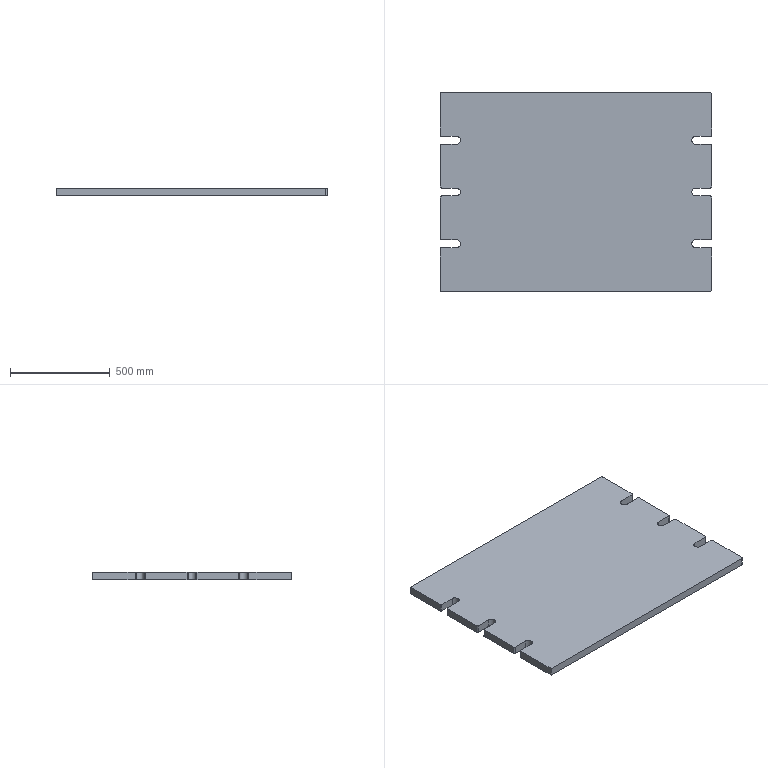Part | SolidWorks | features Fillet 2, Extrusion 1 | 1 solid | 47 faces | box 1360 x 1000 x 40 mm | volume 53476912 mm3 | plane 24 | cylinder 23 | commonest cylinder face diameters 10 x12 40 x9 20 x2
STEP:
#1=CARTESIAN_POINT('',(1260.,760.,40.));
#2=VERTEX_POINT('',#1);
#3=CARTESIAN_POINT('',(1280.,780.,40.));
#4=VERTEX_POINT('',#3);
#5=CARTESIAN_POINT('',(1280.,760.,40.));
#6=DIRECTION('',(0.,0.,-1.));
#7=DIRECTION('',(1.,0.,0.));
#8=AXIS2_PLACEMENT_3D('',#5,#6,#7);
#9=CIRCLE('',#8,20.);
#10=EDGE_CURVE('',#2,#4,#9,.T.);
#11=ORIENTED_EDGE('',*,*,#10,.F.);
#12=CARTESIAN_POINT('',(1260.,760.,0.));
#13=VERTEX_POINT('',#12);
#14=CARTESIAN_POINT('',(1260.,760.,40.));
#15=DIRECTION('',(0.,0.,-1.));
#16=VECTOR('',#15,1000.);
#17=LINE('',#14,#16);
#18=EDGE_CURVE('',#2,#13,#17,.T.);
#19=ORIENTED_EDGE('',*,*,#18,.T.);
#20=CARTESIAN_POINT('',(1280.,780.,0.));
#21=VERTEX_POINT('',#20);
#22=CARTESIAN_POINT('',(1280.,760.,0.));
#23=DIRECTION('',(0.,0.,-1.));
#24=DIRECTION('',(1.,0.,0.));
#25=AXIS2_PLACEMENT_3D('',#22,#23,#24);
#26=CIRCLE('',#25,20.);
#27=EDGE_CURVE('',#13,#21,#26,.T.);
#28=ORIENTED_EDGE('',*,*,#27,.T.);
#29=CARTESIAN_POINT('',(1280.,780.,40.));
#30=DIRECTION('',(0.,0.,-1.));
#31=VECTOR('',#30,1000.);
#32=LINE('',#29,#31);
#33=EDGE_CURVE('',#4,#21,#32,.T.);
#34=ORIENTED_EDGE('',*,*,#33,.F.);
#35=EDGE_LOOP('',(#11,#19,#28,#34));
#36=FACE_OUTER_BOUND('',#35,.T.);
#37=CARTESIAN_POINT('',(1280.,760.,40.));
#38=DIRECTION('',(0.,0.,-1.));
#39=DIRECTION('',(-1.,0.,0.));
#40=AXIS2_PLACEMENT_3D('',#37,#38,#39);
#41=CYLINDRICAL_SURFACE('',#40,20.);
#42=ADVANCED_FACE('',(#36),#41,.F.);
#43=CARTESIAN_POINT('',(1260.,500.,40.));
#44=VERTEX_POINT('',#43);
#45=CARTESIAN_POINT('',(1280.,520.,40.));
#46=VERTEX_POINT('',#45);
#47=CARTESIAN_POINT('',(1280.,500.,40.));
#48=DIRECTION('',(0.,0.,-1.));
#49=DIRECTION('',(1.,0.,0.));
#50=AXIS2_PLACEMENT_3D('',#47,#48,#49);
#51=CIRCLE('',#50,20.);
#52=EDGE_CURVE('',#44,#46,#51,.T.);
#53=ORIENTED_EDGE('',*,*,#52,.F.);
#54=CARTESIAN_POINT('',(1260.,500.,0.));
#55=VERTEX_POINT('',#54);
#56=CARTESIAN_POINT('',(1260.,500.,40.));
#57=DIRECTION('',(0.,0.,-1.));
#58=VECTOR('',#57,1000.);
#59=LINE('',#56,#58);
#60=EDGE_CURVE('',#44,#55,#59,.T.);
#61=ORIENTED_EDGE('',*,*,#60,.T.);
#62=CARTESIAN_POINT('',(1280.,520.,0.));
#63=VERTEX_POINT('',#62);
#64=CARTESIAN_POINT('',(1280.,500.,0.));
#65=DIRECTION('',(0.,0.,-1.));
#66=DIRECTION('',(1.,0.,0.));
#67=AXIS2_PLACEMENT_3D('',#64,#65,#66);
#68=CIRCLE('',#67,20.);
#69=EDGE_CURVE('',#55,#63,#68,.T.);
#70=ORIENTED_EDGE('',*,*,#69,.T.);
#71=CARTESIAN_POINT('',(1280.,520.,40.));
#72=DIRECTION('',(0.,0.,-1.));
#73=VECTOR('',#72,1000.);
#74=LINE('',#71,#73);
#75=EDGE_CURVE('',#46,#63,#74,.T.);
#76=ORIENTED_EDGE('',*,*,#75,.F.);
#77=EDGE_LOOP('',(#53,#61,#70,#76));
#78=FACE_OUTER_BOUND('',#77,.T.);
#79=CARTESIAN_POINT('',(1280.,500.,40.));
#80=DIRECTION('',(0.,0.,-1.));
#81=DIRECTION('',(-1.,0.,0.));
#82=AXIS2_PLACEMENT_3D('',#79,#80,#81);
#83=CYLINDRICAL_SURFACE('',#82,20.);
#84=ADVANCED_FACE('',(#78),#83,.F.);
#85=CARTESIAN_POINT('',(1260.,240.,40.));
#86=VERTEX_POINT('',#85);
#87=CARTESIAN_POINT('',(1280.,260.,40.));
#88=VERTEX_POINT('',#87);
#89=CARTESIAN_POINT('',(1280.,240.,40.));
#90=DIRECTION('',(0.,0.,-1.));
#91=DIRECTION('',(1.,0.,0.));
#92=AXIS2_PLACEMENT_3D('',#89,#90,#91);
#93=CIRCLE('',#92,20.);
#94=EDGE_CURVE('',#86,#88,#93,.T.);
#95=ORIENTED_EDGE('',*,*,#94,.F.);
#96=CARTESIAN_POINT('',(1260.,240.,0.));
#97=VERTEX_POINT('',#96);
#98=CARTESIAN_POINT('',(1260.,240.,40.));
#99=DIRECTION('',(0.,0.,-1.));
#100=VECTOR('',#99,1000.);
#101=LINE('',#98,#100);
#102=EDGE_CURVE('',#86,#97,#101,.T.);
#103=ORIENTED_EDGE('',*,*,#102,.T.);
#104=CARTESIAN_POINT('',(1280.,260.,0.));
#105=VERTEX_POINT('',#104);
#106=CARTESIAN_POINT('',(1280.,240.,0.));
#107=DIRECTION('',(0.,0.,-1.));
#108=DIRECTION('',(1.,0.,0.));
#109=AXIS2_PLACEMENT_3D('',#106,#107,#108);
#110=CIRCLE('',#109,20.);
#111=EDGE_CURVE('',#97,#105,#110,.T.);
#112=ORIENTED_EDGE('',*,*,#111,.T.);
#113=CARTESIAN_POINT('',(1280.,260.,40.));
#114=DIRECTION('',(0.,0.,-1.));
#115=VECTOR('',#114,1000.);
#116=LINE('',#113,#115);
#117=EDGE_CURVE('',#88,#105,#116,.T.);
#118=ORIENTED_EDGE('',*,*,#117,.F.);
#119=EDGE_LOOP('',(#95,#103,#112,#118));
#120=FACE_OUTER_BOUND('',#119,.T.);
#121=CARTESIAN_POINT('',(1280.,240.,40.));
#122=DIRECTION('',(0.,0.,-1.));
#123=DIRECTION('',(-1.,0.,0.));
#124=AXIS2_PLACEMENT_3D('',#121,#122,#123);
#125=CYLINDRICAL_SURFACE('',#124,20.);
#126=ADVANCED_FACE('',(#120),#125,.F.);
#127=CARTESIAN_POINT('',(0.,215.,40.));
#128=VERTEX_POINT('',#127);
#129=CARTESIAN_POINT('',(0.,0.,40.));
#130=VERTEX_POINT('',#129);
#131=CARTESIAN_POINT('',(0.,0.,40.));
#132=DIRECTION('',(0.,-1.,0.));
#133=VECTOR('',#132,1000.);
#134=LINE('',#131,#133);
#135=EDGE_CURVE('',#128,#130,#134,.T.);
#136=ORIENTED_EDGE('',*,*,#135,.F.);
#137=CARTESIAN_POINT('',(0.,215.,0.));
#138=VERTEX_POINT('',#137);
#139=CARTESIAN_POINT('',(0.,215.,40.));
#140=DIRECTION('',(0.,0.,-1.));
#141=VECTOR('',#140,1000.);
#142=LINE('',#139,#141);
#143=EDGE_CURVE('',#128,#138,#142,.T.);
#144=ORIENTED_EDGE('',*,*,#143,.T.);
#145=CARTESIAN_POINT('',(0.,0.,0.));
#146=VERTEX_POINT('',#145);
#147=CARTESIAN_POINT('',(0.,0.,0.));
#148=DIRECTION('',(0.,-1.,0.));
#149=VECTOR('',#148,1000.);
#150=LINE('',#147,#149);
#151=EDGE_CURVE('',#138,#146,#150,.T.);
#152=ORIENTED_EDGE('',*,*,#151,.T.);
#153=CARTESIAN_POINT('',(0.,0.,40.));
#154=DIRECTION('',(0.,0.,-1.));
#155=VECTOR('',#154,1000.);
#156=LINE('',#153,#155);
#157=EDGE_CURVE('',#130,#146,#156,.T.);
#158=ORIENTED_EDGE('',*,*,#157,.F.);
#159=EDGE_LOOP('',(#136,#144,#152,#158));
#160=FACE_OUTER_BOUND('',#159,.T.);
#161=CARTESIAN_POINT('',(0.,0.,40.));
#162=DIRECTION('',(1.,0.,0.));
#163=DIRECTION('',(0.,1.,0.));
#164=AXIS2_PLACEMENT_3D('',#161,#162,#163);
#165=PLANE('',#164);
#166=ADVANCED_FACE('',(#160),#165,.F.);
#167=CARTESIAN_POINT('',(1350.,0.,0.));
#168=VERTEX_POINT('',#167);
#169=CARTESIAN_POINT('',(0.,0.,0.));
#170=DIRECTION('',(1.,0.,0.));
#171=VECTOR('',#170,1000.);
#172=LINE('',#169,#171);
#173=EDGE_CURVE('',#146,#168,#172,.T.);
#174=ORIENTED_EDGE('',*,*,#173,.T.);
#175=CARTESIAN_POINT('',(1350.,0.,40.));
#176=VERTEX_POINT('',#175);
#177=CARTESIAN_POINT('',(1350.,0.,40.));
#178=DIRECTION('',(0.,0.,1.));
#179=VECTOR('',#178,1000.);
#180=LINE('',#177,#179);
#181=EDGE_CURVE('',#168,#176,#180,.T.);
#182=ORIENTED_EDGE('',*,*,#181,.T.);
#183=CARTESIAN_POINT('',(0.,0.,40.));
#184=DIRECTION('',(1.,0.,0.));
#185=VECTOR('',#184,1000.);
#186=LINE('',#183,#185);
#187=EDGE_CURVE('',#130,#176,#186,.T.);
#188=ORIENTED_EDGE('',*,*,#187,.F.);
#189=ORIENTED_EDGE('',*,*,#157,.T.);
#190=EDGE_LOOP('',(#174,#182,#188,#189));
#191=FACE_OUTER_BOUND('',#190,.T.);
#192=CARTESIAN_POINT('',(0.,0.,40.));
#193=DIRECTION('',(0.,1.,0.));
#194=DIRECTION('',(0.,0.,1.));
#195=AXIS2_PLACEMENT_3D('',#192,#193,#194);
#196=PLANE('',#195);
#197=ADVANCED_FACE('',(#191),#196,.F.);
#198=CARTESIAN_POINT('',(1360.,10.,40.));
#199=VERTEX_POINT('',#198);
#200=CARTESIAN_POINT('',(1360.,215.,40.));
#201=VERTEX_POINT('',#200);
#202=CARTESIAN_POINT('',(1360.,0.,40.));
#203=DIRECTION('',(0.,1.,0.));
#204=VECTOR('',#203,1000.);
#205=LINE('',#202,#204);
#206=EDGE_CURVE('',#199,#201,#205,.T.);
#207=ORIENTED_EDGE('',*,*,#206,.F.);
#208=CARTESIAN_POINT('',(1360.,10.,0.));
#209=VERTEX_POINT('',#208);
#210=CARTESIAN_POINT('',(1360.,10.,40.));
#211=DIRECTION('',(0.,0.,-1.));
#212=VECTOR('',#211,1000.);
#213=LINE('',#210,#212);
#214=EDGE_CURVE('',#199,#209,#213,.T.);
#215=ORIENTED_EDGE('',*,*,#214,.T.);
#216=CARTESIAN_POINT('',(1360.,215.,0.));
#217=VERTEX_POINT('',#216);
#218=CARTESIAN_POINT('',(1360.,0.,0.));
#219=DIRECTION('',(0.,1.,0.));
#220=VECTOR('',#219,1000.);
#221=LINE('',#218,#220);
#222=EDGE_CURVE('',#209,#217,#221,.T.);
#223=ORIENTED_EDGE('',*,*,#222,.T.);
#224=CARTESIAN_POINT('',(1360.,215.,40.));
#225=DIRECTION('',(0.,0.,1.));
#226=VECTOR('',#225,1000.);
#227=LINE('',#224,#226);
#228=EDGE_CURVE('',#217,#201,#227,.T.);
#229=ORIENTED_EDGE('',*,*,#228,.T.);
#230=EDGE_LOOP('',(#207,#215,#223,#229));
#231=FACE_OUTER_BOUND('',#230,.T.);
#232=CARTESIAN_POINT('',(1360.,0.,40.));
#233=DIRECTION('',(-1.,0.,0.));
#234=DIRECTION('',(0.,0.,1.));
#235=AXIS2_PLACEMENT_3D('',#232,#233,#234);
#236=PLANE('',#235);
#237=ADVANCED_FACE('',(#231),#236,.F.);
#238=CARTESIAN_POINT('',(1355.,220.,40.));
#239=VERTEX_POINT('',#238);
#240=CARTESIAN_POINT('',(1280.,220.,40.));
#241=VERTEX_POINT('',#240);
#242=CARTESIAN_POINT('',(1280.,220.,40.));
#243=DIRECTION('',(-1.,0.,0.));
#244=VECTOR('',#243,1000.);
#245=LINE('',#242,#244);
#246=EDGE_CURVE('',#239,#241,#245,.T.);
#247=ORIENTED_EDGE('',*,*,#246,.F.);
#248=CARTESIAN_POINT('',(1355.,220.,0.));
#249=VERTEX_POINT('',#248);
#250=CARTESIAN_POINT('',(1355.,220.,40.));
#251=DIRECTION('',(0.,0.,-1.));
#252=VECTOR('',#251,1000.);
#253=LINE('',#250,#252);
#254=EDGE_CURVE('',#239,#249,#253,.T.);
#255=ORIENTED_EDGE('',*,*,#254,.T.);
#256=CARTESIAN_POINT('',(1280.,220.,0.));
#257=VERTEX_POINT('',#256);
#258=CARTESIAN_POINT('',(1280.,220.,0.));
#259=DIRECTION('',(-1.,0.,0.));
#260=VECTOR('',#259,1000.);
#261=LINE('',#258,#260);
#262=EDGE_CURVE('',#249,#257,#261,.T.);
#263=ORIENTED_EDGE('',*,*,#262,.T.);
#264=CARTESIAN_POINT('',(1280.,220.,40.));
#265=DIRECTION('',(0.,0.,-1.));
#266=VECTOR('',#265,1000.);
#267=LINE('',#264,#266);
#268=EDGE_CURVE('',#241,#257,#267,.T.);
#269=ORIENTED_EDGE('',*,*,#268,.F.);
#270=EDGE_LOOP('',(#247,#255,#263,#269));
#271=FACE_OUTER_BOUND('',#270,.T.);
#272=CARTESIAN_POINT('',(1280.,220.,40.));
#273=DIRECTION('',(0.,-1.,0.));
#274=DIRECTION('',(1.,0.,0.));
#275=AXIS2_PLACEMENT_3D('',#272,#273,#274);
#276=PLANE('',#275);
#277=ADVANCED_FACE('',(#271),#276,.F.);
#278=ORIENTED_EDGE('',*,*,#102,.F.);
#279=CARTESIAN_POINT('',(1280.,240.,40.));
#280=DIRECTION('',(0.,0.,-1.));
#281=DIRECTION('',(1.,0.,0.));
#282=AXIS2_PLACEMENT_3D('',#279,#280,#281);
#283=CIRCLE('',#282,20.);
#284=EDGE_CURVE('',#241,#86,#283,.T.);
#285=ORIENTED_EDGE('',*,*,#284,.F.);
#286=ORIENTED_EDGE('',*,*,#268,.T.);
#287=CARTESIAN_POINT('',(1280.,240.,0.));
#288=DIRECTION('',(0.,0.,-1.));
#289=DIRECTION('',(1.,0.,0.));
#290=AXIS2_PLACEMENT_3D('',#287,#288,#289);
#291=CIRCLE('',#290,20.);
#292=EDGE_CURVE('',#257,#97,#291,.T.);
#293=ORIENTED_EDGE('',*,*,#292,.T.);
#294=EDGE_LOOP('',(#278,#285,#286,#293));
#295=FACE_OUTER_BOUND('',#294,.T.);
#296=CARTESIAN_POINT('',(1280.,240.,40.));
#297=DIRECTION('',(0.,0.,-1.));
#298=DIRECTION('',(-1.,0.,0.));
#299=AXIS2_PLACEMENT_3D('',#296,#297,#298);
#300=CYLINDRICAL_SURFACE('',#299,20.);
#301=ADVANCED_FACE('',(#295),#300,.F.);
#302=CARTESIAN_POINT('',(1355.,260.,0.));
#303=VERTEX_POINT('',#302);
#304=CARTESIAN_POINT('',(1360.,260.,0.));
#305=DIRECTION('',(1.,0.,0.));
#306=VECTOR('',#305,1000.);
#307=LINE('',#304,#306);
#308=EDGE_CURVE('',#105,#303,#307,.T.);
#309=ORIENTED_EDGE('',*,*,#308,.T.);
#310=CARTESIAN_POINT('',(1355.,260.,40.));
#311=VERTEX_POINT('',#310);
#312=CARTESIAN_POINT('',(1355.,260.,40.));
#313=DIRECTION('',(0.,0.,1.));
#314=VECTOR('',#313,1000.);
#315=LINE('',#312,#314);
#316=EDGE_CURVE('',#303,#311,#315,.T.);
#317=ORIENTED_EDGE('',*,*,#316,.T.);
#318=CARTESIAN_POINT('',(1360.,260.,40.));
#319=DIRECTION('',(1.,0.,0.));
#320=VECTOR('',#319,1000.);
#321=LINE('',#318,#320);
#322=EDGE_CURVE('',#88,#311,#321,.T.);
#323=ORIENTED_EDGE('',*,*,#322,.F.);
#324=ORIENTED_EDGE('',*,*,#117,.T.);
#325=EDGE_LOOP('',(#309,#317,#323,#324));
#326=FACE_OUTER_BOUND('',#325,.T.);
#327=CARTESIAN_POINT('',(1360.,260.,40.));
#328=DIRECTION('',(0.,1.,0.));
#329=DIRECTION('',(0.,0.,1.));
#330=AXIS2_PLACEMENT_3D('',#327,#328,#329);
#331=PLANE('',#330);
#332=ADVANCED_FACE('',(#326),#331,.F.);
#333=CARTESIAN_POINT('',(1360.,265.,0.));
#334=VERTEX_POINT('',#333);
#335=CARTESIAN_POINT('',(1360.,475.,0.));
#336=VERTEX_POINT('',#335);
#337=CARTESIAN_POINT('',(1360.,260.,0.));
#338=DIRECTION('',(0.,1.,0.));
#339=VECTOR('',#338,1000.);
#340=LINE('',#337,#339);
#341=EDGE_CURVE('',#334,#336,#340,.T.);
#342=ORIENTED_EDGE('',*,*,#341,.T.);
#343=CARTESIAN_POINT('',(1360.,475.,40.));
#344=VERTEX_POINT('',#343);
#345=CARTESIAN_POINT('',(1360.,475.,40.));
#346=DIRECTION('',(0.,0.,1.));
#347=VECTOR('',#346,1000.);
#348=LINE('',#345,#347);
#349=EDGE_CURVE('',#336,#344,#348,.T.);
#350=ORIENTED_EDGE('',*,*,#349,.T.);
#351=CARTESIAN_POINT('',(1360.,265.,40.));
#352=VERTEX_POINT('',#351);
#353=CARTESIAN_POINT('',(1360.,260.,40.));
#354=DIRECTION('',(0.,1.,0.));
#355=VECTOR('',#354,1000.);
#356=LINE('',#353,#355);
#357=EDGE_CURVE('',#352,#344,#356,.T.);
#358=ORIENTED_EDGE('',*,*,#357,.F.);
#359=CARTESIAN_POINT('',(1360.,265.,40.));
#360=DIRECTION('',(0.,0.,-1.));
#361=VECTOR('',#360,1000.);
#362=LINE('',#359,#361);
#363=EDGE_CURVE('',#352,#334,#362,.T.);
#364=ORIENTED_EDGE('',*,*,#363,.T.);
#365=EDGE_LOOP('',(#342,#350,#358,#364));
#366=FACE_OUTER_BOUND('',#365,.T.);
#367=CARTESIAN_POINT('',(1360.,260.,40.));
#368=DIRECTION('',(-1.,0.,0.));
#369=DIRECTION('',(0.,0.,1.));
#370=AXIS2_PLACEMENT_3D('',#367,#368,#369);
#371=PLANE('',#370);
#372=ADVANCED_FACE('',(#366),#371,.F.);
#373=CARTESIAN_POINT('',(1355.,480.,40.));
#374=VERTEX_POINT('',#373);
#375=CARTESIAN_POINT('',(1280.,480.,40.));
#376=VERTEX_POINT('',#375);
#377=CARTESIAN_POINT('',(1280.,480.,40.));
#378=DIRECTION('',(-1.,0.,0.));
#379=VECTOR('',#378,1000.);
#380=LINE('',#377,#379);
#381=EDGE_CURVE('',#374,#376,#380,.T.);
#382=ORIENTED_EDGE('',*,*,#381,.F.);
#383=CARTESIAN_POINT('',(1355.,480.,0.));
#384=VERTEX_POINT('',#383);
#385=CARTESIAN_POINT('',(1355.,480.,40.));
#386=DIRECTION('',(0.,0.,-1.));
#387=VECTOR('',#386,1000.);
#388=LINE('',#385,#387);
#389=EDGE_CURVE('',#374,#384,#388,.T.);
#390=ORIENTED_EDGE('',*,*,#389,.T.);
#391=CARTESIAN_POINT('',(1280.,480.,0.));
#392=VERTEX_POINT('',#391);
#393=CARTESIAN_POINT('',(1280.,480.,0.));
#394=DIRECTION('',(-1.,0.,0.));
#395=VECTOR('',#394,1000.);
#396=LINE('',#393,#395);
#397=EDGE_CURVE('',#384,#392,#396,.T.);
#398=ORIENTED_EDGE('',*,*,#397,.T.);
#399=CARTESIAN_POINT('',(1280.,480.,40.));
#400=DIRECTION('',(0.,0.,-1.));
#401=VECTOR('',#400,1000.);
#402=LINE('',#399,#401);
#403=EDGE_CURVE('',#376,#392,#402,.T.);
#404=ORIENTED_EDGE('',*,*,#403,.F.);
#405=EDGE_LOOP('',(#382,#390,#398,#404));
#406=FACE_OUTER_BOUND('',#405,.T.);
#407=CARTESIAN_POINT('',(1280.,480.,40.));
#408=DIRECTION('',(0.,-1.,0.));
#409=DIRECTION('',(1.,0.,0.));
#410=AXIS2_PLACEMENT_3D('',#407,#408,#409);
#411=PLANE('',#410);
#412=ADVANCED_FACE('',(#406),#411,.F.);
#413=ORIENTED_EDGE('',*,*,#60,.F.);
#414=CARTESIAN_POINT('',(1280.,500.,40.));
#415=DIRECTION('',(0.,0.,-1.));
#416=DIRECTION('',(1.,0.,0.));
#417=AXIS2_PLACEMENT_3D('',#414,#415,#416);
#418=CIRCLE('',#417,20.);
#419=EDGE_CURVE('',#376,#44,#418,.T.);
#420=ORIENTED_EDGE('',*,*,#419,.F.);
#421=ORIENTED_EDGE('',*,*,#403,.T.);
#422=CARTESIAN_POINT('',(1280.,500.,0.));
#423=DIRECTION('',(0.,0.,-1.));
#424=DIRECTION('',(1.,0.,0.));
#425=AXIS2_PLACEMENT_3D('',#422,#423,#424);
#426=CIRCLE('',#425,20.);
#427=EDGE_CURVE('',#392,#55,#426,.T.);
#428=ORIENTED_EDGE('',*,*,#427,.T.);
#429=EDGE_LOOP('',(#413,#420,#421,#428));
#430=FACE_OUTER_BOUND('',#429,.T.);
#431=CARTESIAN_POINT('',(1280.,500.,40.));
#432=DIRECTION('',(0.,0.,-1.));
#433=DIRECTION('',(-1.,0.,0.));
#434=AXIS2_PLACEMENT_3D('',#431,#432,#433);
#435=CYLINDRICAL_SURFACE('',#434,20.);
#436=ADVANCED_FACE('',(#430),#435,.F.);
#437=CARTESIAN_POINT('',(1355.,520.,0.));
#438=VERTEX_POINT('',#437);
#439=CARTESIAN_POINT('',(1360.,520.,0.));
#440=DIRECTION('',(1.,0.,0.));
#441=VECTOR('',#440,1000.);
#442=LINE('',#439,#441);
#443=EDGE_CURVE('',#63,#438,#442,.T.);
#444=ORIENTED_EDGE('',*,*,#443,.T.);
#445=CARTESIAN_POINT('',(1355.,520.,40.));
#446=VERTEX_POINT('',#445);
#447=CARTESIAN_POINT('',(1355.,520.,40.));
#448=DIRECTION('',(0.,0.,1.));
#449=VECTOR('',#448,1000.);
#450=LINE('',#447,#449);
#451=EDGE_CURVE('',#438,#446,#450,.T.);
#452=ORIENTED_EDGE('',*,*,#451,.T.);
#453=CARTESIAN_POINT('',(1360.,520.,40.));
#454=DIRECTION('',(1.,0.,0.));
#455=VECTOR('',#454,1000.);
#456=LINE('',#453,#455);
#457=EDGE_CURVE('',#46,#446,#456,.T.);
#458=ORIENTED_EDGE('',*,*,#457,.F.);
#459=ORIENTED_EDGE('',*,*,#75,.T.);
#460=EDGE_LOOP('',(#444,#452,#458,#459));
#461=FACE_OUTER_BOUND('',#460,.T.);
#462=CARTESIAN_POINT('',(1360.,520.,40.));
#463=DIRECTION('',(0.,1.,0.));
#464=DIRECTION('',(0.,0.,1.));
#465=AXIS2_PLACEMENT_3D('',#462,#463,#464);
#466=PLANE('',#465);
#467=ADVANCED_FACE('',(#461),#466,.F.);
#468=CARTESIAN_POINT('',(1360.,525.,0.));
#469=VERTEX_POINT('',#468);
#470=CARTESIAN_POINT('',(1360.,735.,0.));
#471=VERTEX_POINT('',#470);
#472=CARTESIAN_POINT('',(1360.,520.,0.));
#473=DIRECTION('',(0.,1.,0.));
#474=VECTOR('',#473,1000.);
#475=LINE('',#472,#474);
#476=EDGE_CURVE('',#469,#471,#475,.T.);
#477=ORIENTED_EDGE('',*,*,#476,.T.);
#478=CARTESIAN_POINT('',(1360.,735.,40.));
#479=VERTEX_POINT('',#478);
#480=CARTESIAN_POINT('',(1360.,735.,40.));
#481=DIRECTION('',(0.,0.,1.));
#482=VECTOR('',#481,1000.);
#483=LINE('',#480,#482);
#484=EDGE_CURVE('',#471,#479,#483,.T.);
#485=ORIENTED_EDGE('',*,*,#484,.T.);
#486=CARTESIAN_POINT('',(1360.,525.,40.));
#487=VERTEX_POINT('',#486);
#488=CARTESIAN_POINT('',(1360.,520.,40.));
#489=DIRECTION('',(0.,1.,0.));
#490=VECTOR('',#489,1000.);
#491=LINE('',#488,#490);
#492=EDGE_CURVE('',#487,#479,#491,.T.);
#493=ORIENTED_EDGE('',*,*,#492,.F.);
#494=CARTESIAN_POINT('',(1360.,525.,40.));
#495=DIRECTION('',(0.,0.,-1.));
#496=VECTOR('',#495,1000.);
#497=LINE('',#494,#496);
#498=EDGE_CURVE('',#487,#469,#497,.T.);
#499=ORIENTED_EDGE('',*,*,#498,.T.);
#500=EDGE_LOOP('',(#477,#485,#493,#499));
#501=FACE_OUTER_BOUND('',#500,.T.);
#502=CARTESIAN_POINT('',(1360.,520.,40.));
#503=DIRECTION('',(-1.,0.,0.));
#504=DIRECTION('',(0.,0.,1.));
#505=AXIS2_PLACEMENT_3D('',#502,#503,#504);
#506=PLANE('',#505);
#507=ADVANCED_FACE('',(#501),#506,.F.);
#508=CARTESIAN_POINT('',(1355.,740.,40.));
#509=VERTEX_POINT('',#508);
#510=CARTESIAN_POINT('',(1280.,740.,40.));
#511=VERTEX_POINT('',#510);
#512=CARTESIAN_POINT('',(1280.,740.,40.));
#513=DIRECTION('',(-1.,0.,0.));
#514=VECTOR('',#513,1000.);
#515=LINE('',#512,#514);
#516=EDGE_CURVE('',#509,#511,#515,.T.);
#517=ORIENTED_EDGE('',*,*,#516,.F.);
#518=CARTESIAN_POINT('',(1355.,740.,0.));
#519=VERTEX_POINT('',#518);
#520=CARTESIAN_POINT('',(1355.,740.,40.));
#521=DIRECTION('',(0.,0.,-1.));
#522=VECTOR('',#521,1000.);
#523=LINE('',#520,#522);
#524=EDGE_CURVE('',#509,#519,#523,.T.);
#525=ORIENTED_EDGE('',*,*,#524,.T.);
#526=CARTESIAN_POINT('',(1280.,740.,0.));
#527=VERTEX_POINT('',#526);
#528=CARTESIAN_POINT('',(1280.,740.,0.));
#529=DIRECTION('',(-1.,0.,0.));
#530=VECTOR('',#529,1000.);
#531=LINE('',#528,#530);
#532=EDGE_CURVE('',#519,#527,#531,.T.);
#533=ORIENTED_EDGE('',*,*,#532,.T.);
#534=CARTESIAN_POINT('',(1280.,740.,40.));
#535=DIRECTION('',(0.,0.,-1.));
#536=VECTOR('',#535,1000.);
#537=LINE('',#534,#536);
#538=EDGE_CURVE('',#511,#527,#537,.T.);
#539=ORIENTED_EDGE('',*,*,#538,.F.);
#540=EDGE_LOOP('',(#517,#525,#533,#539));
#541=FACE_OUTER_BOUND('',#540,.T.);
#542=CARTESIAN_POINT('',(1280.,740.,40.));
#543=DIRECTION('',(0.,-1.,0.));
#544=DIRECTION('',(1.,0.,0.));
#545=AXIS2_PLACEMENT_3D('',#542,#543,#544);
#546=PLANE('',#545);
#547=ADVANCED_FACE('',(#541),#546,.F.);
#548=ORIENTED_EDGE('',*,*,#18,.F.);
#549=CARTESIAN_POINT('',(1280.,760.,40.));
#550=DIRECTION('',(0.,0.,-1.));
#551=DIRECTION('',(1.,0.,0.));
#552=AXIS2_PLACEMENT_3D('',#549,#550,#551);
#553=CIRCLE('',#552,20.);
#554=EDGE_CURVE('',#511,#2,#553,.T.);
#555=ORIENTED_EDGE('',*,*,#554,.F.);
#556=ORIENTED_EDGE('',*,*,#538,.T.);
#557=CARTESIAN_POINT('',(1280.,760.,0.));
#558=DIRECTION('',(0.,0.,-1.));
#559=DIRECTION('',(1.,0.,0.));
#560=AXIS2_PLACEMENT_3D('',#557,#558,#559);
#561=CIRCLE('',#560,20.);
#562=EDGE_CURVE('',#527,#13,#561,.T.);
#563=ORIENTED_EDGE('',*,*,#562,.T.);
#564=EDGE_LOOP('',(#548,#555,#556,#563));
#565=FACE_OUTER_BOUND('',#564,.T.);
#566=CARTESIAN_POINT('',(1280.,760.,40.));
#567=DIRECTION('',(0.,0.,-1.));
#568=DIRECTION('',(-1.,0.,0.));
#569=AXIS2_PLACEMENT_3D('',#566,#567,#568);
#570=CYLINDRICAL_SURFACE('',#569,20.);
#571=ADVANCED_FACE('',(#565),#570,.F.);
#572=CARTESIAN_POINT('',(1355.,780.,0.));
#573=VERTEX_POINT('',#572);
#574=CARTESIAN_POINT('',(1360.,780.,0.));
#575=DIRECTION('',(1.,0.,0.));
#576=VECTOR('',#575,1000.);
#577=LINE('',#574,#576);
#578=EDGE_CURVE('',#21,#573,#577,.T.);
#579=ORIENTED_EDGE('',*,*,#578,.T.);
#580=CARTESIAN_POINT('',(1355.,780.,40.));
#581=VERTEX_POINT('',#580);
#582=CARTESIAN_POINT('',(1355.,780.,40.));
#583=DIRECTION('',(0.,0.,1.));
#584=VECTOR('',#583,1000.);
#585=LINE('',#582,#584);
#586=EDGE_CURVE('',#573,#581,#585,.T.);
#587=ORIENTED_EDGE('',*,*,#586,.T.);
#588=CARTESIAN_POINT('',(1360.,780.,40.));
#589=DIRECTION('',(1.,0.,0.));
#590=VECTOR('',#589,1000.);
#591=LINE('',#588,#590);
#592=EDGE_CURVE('',#4,#581,#591,.T.);
#593=ORIENTED_EDGE('',*,*,#592,.F.);
#594=ORIENTED_EDGE('',*,*,#33,.T.);
#595=EDGE_LOOP('',(#579,#587,#593,#594));
#596=FACE_OUTER_BOUND('',#595,.T.);
#597=CARTESIAN_POINT('',(1360.,780.,40.));
#598=DIRECTION('',(0.,1.,0.));
#599=DIRECTION('',(0.,0.,1.));
#600=AXIS2_PLACEMENT_3D('',#597,#598,#599);
#601=PLANE('',#600);
#602=ADVANCED_FACE('',(#596),#601,.F.);
#603=CARTESIAN_POINT('',(1360.,785.,0.));
#604=VERTEX_POINT('',#603);
#605=CARTESIAN_POINT('',(1360.,990.,0.));
#606=VERTEX_POINT('',#605);
#607=CARTESIAN_POINT('',(1360.,780.,0.));
#608=DIRECTION('',(0.,1.,0.));
#609=VECTOR('',#608,1000.);
#610=LINE('',#607,#609);
#611=EDGE_CURVE('',#604,#606,#610,.T.);
#612=ORIENTED_EDGE('',*,*,#611,.T.);
#613=CARTESIAN_POINT('',(1360.,990.,40.));
#614=VERTEX_POINT('',#613);
#615=CARTESIAN_POINT('',(1360.,990.,40.));
#616=DIRECTION('',(0.,0.,1.));
#617=VECTOR('',#616,1000.);
#618=LINE('',#615,#617);
#619=EDGE_CURVE('',#606,#614,#618,.T.);
#620=ORIENTED_EDGE('',*,*,#619,.T.);
#621=CARTESIAN_POINT('',(1360.,785.,40.));
#622=VERTEX_POINT('',#621);
#623=CARTESIAN_POINT('',(1360.,780.,40.));
#624=DIRECTION('',(0.,1.,0.));
#625=VECTOR('',#624,1000.);
#626=LINE('',#623,#625);
#627=EDGE_CURVE('',#622,#614,#626,.T.);
#628=ORIENTED_EDGE('',*,*,#627,.F.);
#629=CARTESIAN_POINT('',(1360.,785.,40.));
#630=DIRECTION('',(0.,0.,-1.));
#631=VECTOR('',#630,1000.);
#632=LINE('',#629,#631);
#633=EDGE_CURVE('',#622,#604,#632,.T.);
#634=ORIENTED_EDGE('',*,*,#633,.T.);
#635=EDGE_LOOP('',(#612,#620,#628,#634));
#636=FACE_OUTER_BOUND('',#635,.T.);
#637=CARTESIAN_POINT('',(1360.,780.,40.));
#638=DIRECTION('',(-1.,0.,0.));
#639=DIRECTION('',(0.,0.,1.));
#640=AXIS2_PLACEMENT_3D('',#637,#638,#639);
#641=PLANE('',#640);
#642=ADVANCED_FACE('',(#636),#641,.F.);
#643=CARTESIAN_POINT('',(1350.,1000.,40.));
#644=VERTEX_POINT('',#643);
#645=CARTESIAN_POINT('',(0.,1000.,40.));
#646=VERTEX_POINT('',#645);
#647=CARTESIAN_POINT('',(0.,1000.,40.));
#648=DIRECTION('',(-1.,0.,0.));
#649=VECTOR('',#648,1000.);
#650=LINE('',#647,#649);
#651=EDGE_CURVE('',#644,#646,#650,.T.);
#652=ORIENTED_EDGE('',*,*,#651,.F.);
#653=CARTESIAN_POINT('',(1350.,1000.,0.));
#654=VERTEX_POINT('',#653);
#655=CARTESIAN_POINT('',(1350.,1000.,40.));
#656=DIRECTION('',(0.,0.,-1.));
#657=VECTOR('',#656,1000.);
#658=LINE('',#655,#657);
#659=EDGE_CURVE('',#644,#654,#658,.T.);
#660=ORIENTED_EDGE('',*,*,#659,.T.);
#661=CARTESIAN_POINT('',(0.,1000.,0.));
#662=VERTEX_POINT('',#661);
#663=CARTESIAN_POINT('',(0.,1000.,0.));
#664=DIRECTION('',(-1.,0.,0.));
#665=VECTOR('',#664,1000.);
#666=LINE('',#663,#665);
#667=EDGE_CURVE('',#654,#662,#666,.T.);
#668=ORIENTED_EDGE('',*,*,#667,.T.);
#669=CARTESIAN_POINT('',(0.,1000.,40.));
#670=DIRECTION('',(0.,0.,-1.));
#671=VECTOR('',#670,1000.);
#672=LINE('',#669,#671);
#673=EDGE_CURVE('',#646,#662,#672,.T.);
#674=ORIENTED_EDGE('',*,*,#673,.F.);
#675=EDGE_LOOP('',(#652,#660,#668,#674));
#676=FACE_OUTER_BOUND('',#675,.T.);
#677=CARTESIAN_POINT('',(0.,1000.,40.));
#678=DIRECTION('',(0.,-1.,0.));
#679=DIRECTION('',(0.,0.,-1.));
#680=AXIS2_PLACEMENT_3D('',#677,#678,#679);
#681=PLANE('',#680);
#682=ADVANCED_FACE('',(#676),#681,.F.);
#683=CARTESIAN_POINT('',(0.,785.,0.));
#684=VERTEX_POINT('',#683);
#685=CARTESIAN_POINT('',(0.,780.,0.));
#686=DIRECTION('',(0.,-1.,0.));
#687=VECTOR('',#686,1000.);
#688=LINE('',#685,#687);
#689=EDGE_CURVE('',#662,#684,#688,.T.);
#690=ORIENTED_EDGE('',*,*,#689,.T.);
#691=CARTESIAN_POINT('',(0.,785.,40.));
#692=VERTEX_POINT('',#691);
#693=CARTESIAN_POINT('',(0.,785.,40.));
#694=DIRECTION('',(0.,0.,1.));
#695=VECTOR('',#694,1000.);
#696=LINE('',#693,#695);
#697=EDGE_CURVE('',#684,#692,#696,.T.);
#698=ORIENTED_EDGE('',*,*,#697,.T.);
#699=CARTESIAN_POINT('',(0.,780.,40.));
#700=DIRECTION('',(0.,-1.,0.));
#701=VECTOR('',#700,1000.);
#702=LINE('',#699,#701);
#703=EDGE_CURVE('',#646,#692,#702,.T.);
#704=ORIENTED_EDGE('',*,*,#703,.F.);
#705=ORIENTED_EDGE('',*,*,#673,.T.);
#706=EDGE_LOOP('',(#690,#698,#704,#705));
#707=FACE_OUTER_BOUND('',#706,.T.);
#708=CARTESIAN_POINT('',(0.,780.,40.));
#709=DIRECTION('',(1.,0.,0.));
#710=DIRECTION('',(0.,0.,-1.));
#711=AXIS2_PLACEMENT_3D('',#708,#709,#710);
#712=PLANE('',#711);
#713=ADVANCED_FACE('',(#707),#712,.F.);
#714=CARTESIAN_POINT('',(5.,780.,40.));
#715=VERTEX_POINT('',#714);
#716=CARTESIAN_POINT('',(80.,780.,40.));
#717=VERTEX_POINT('',#716);
#718=CARTESIAN_POINT('',(0.,780.,40.));
#719=DIRECTION('',(1.,0.,0.));
#720=VECTOR('',#719,1000.);
#721=LINE('',#718,#720);
#722=EDGE_CURVE('',#715,#717,#721,.T.);
#723=ORIENTED_EDGE('',*,*,#722,.F.);
#724=CARTESIAN_POINT('',(5.,780.,0.));
#725=VERTEX_POINT('',#724);
#726=CARTESIAN_POINT('',(5.,780.,40.));
#727=DIRECTION('',(0.,0.,-1.));
#728=VECTOR('',#727,1000.);
#729=LINE('',#726,#728);
#730=EDGE_CURVE('',#715,#725,#729,.T.);
#731=ORIENTED_EDGE('',*,*,#730,.T.);
#732=CARTESIAN_POINT('',(80.,780.,0.));
#733=VERTEX_POINT('',#732);
#734=CARTESIAN_POINT('',(0.,780.,0.));
#735=DIRECTION('',(1.,0.,0.));
#736=VECTOR('',#735,1000.);
#737=LINE('',#734,#736);
#738=EDGE_CURVE('',#725,#733,#737,.T.);
#739=ORIENTED_EDGE('',*,*,#738,.T.);
#740=CARTESIAN_POINT('',(80.,780.,40.));
#741=DIRECTION('',(0.,0.,-1.));
#742=VECTOR('',#741,1000.);
#743=LINE('',#740,#742);
#744=EDGE_CURVE('',#717,#733,#743,.T.);
#745=ORIENTED_EDGE('',*,*,#744,.F.);
#746=EDGE_LOOP('',(#723,#731,#739,#745));
#747=FACE_OUTER_BOUND('',#746,.T.);
#748=CARTESIAN_POINT('',(0.,780.,40.));
#749=DIRECTION('',(0.,1.,0.));
#750=DIRECTION('',(0.,0.,1.));
#751=AXIS2_PLACEMENT_3D('',#748,#749,#750);
#752=PLANE('',#751);
#753=ADVANCED_FACE('',(#747),#752,.F.);
#754=CARTESIAN_POINT('',(80.,740.,0.));
#755=VERTEX_POINT('',#754);
#756=CARTESIAN_POINT('',(80.,760.,0.));
#757=DIRECTION('',(0.,0.,-1.));
#758=DIRECTION('',(-1.,0.,0.));
#759=AXIS2_PLACEMENT_3D('',#756,#757,#758);
#760=CIRCLE('',#759,20.);
#761=EDGE_CURVE('',#733,#755,#760,.T.);
#762=ORIENTED_EDGE('',*,*,#761,.T.);
#763=CARTESIAN_POINT('',(80.,740.,40.));
#764=VERTEX_POINT('',#763);
#765=CARTESIAN_POINT('',(80.,740.,40.));
#766=DIRECTION('',(0.,0.,-1.));
#767=VECTOR('',#766,1000.);
#768=LINE('',#765,#767);
#769=EDGE_CURVE('',#764,#755,#768,.T.);
#770=ORIENTED_EDGE('',*,*,#769,.F.);
#771=CARTESIAN_POINT('',(80.,760.,40.));
#772=DIRECTION('',(0.,0.,-1.));
#773=DIRECTION('',(-1.,0.,0.));
#774=AXIS2_PLACEMENT_3D('',#771,#772,#773);
#775=CIRCLE('',#774,20.);
#776=EDGE_CURVE('',#717,#764,#775,.T.);
#777=ORIENTED_EDGE('',*,*,#776,.F.);
#778=ORIENTED_EDGE('',*,*,#744,.T.);
#779=EDGE_LOOP('',(#762,#770,#777,#778));
#780=FACE_OUTER_BOUND('',#779,.T.);
#781=CARTESIAN_POINT('',(80.,760.,40.));
#782=DIRECTION('',(0.,0.,-1.));
#783=DIRECTION('',(-1.,0.,0.));
#784=AXIS2_PLACEMENT_3D('',#781,#782,#783);
#785=CYLINDRICAL_SURFACE('',#784,20.);
#786=ADVANCED_FACE('',(#780),#785,.F.);
#787=CARTESIAN_POINT('',(5.,740.,0.));
#788=VERTEX_POINT('',#787);
#789=CARTESIAN_POINT('',(80.,740.,0.));
#790=DIRECTION('',(-1.,0.,0.));
#791=VECTOR('',#790,1000.);
#792=LINE('',#789,#791);
#793=EDGE_CURVE('',#755,#788,#792,.T.);
#794=ORIENTED_EDGE('',*,*,#793,.T.);
#795=CARTESIAN_POINT('',(5.,740.,40.));
#796=VERTEX_POINT('',#795);
#797=CARTESIAN_POINT('',(5.,740.,40.));
#798=DIRECTION('',(0.,0.,1.));
#799=VECTOR('',#798,1000.);
#800=LINE('',#797,#799);
#801=EDGE_CURVE('',#788,#796,#800,.T.);
#802=ORIENTED_EDGE('',*,*,#801,.T.);
#803=CARTESIAN_POINT('',(80.,740.,40.));
#804=DIRECTION('',(-1.,0.,0.));
#805=VECTOR('',#804,1000.);
#806=LINE('',#803,#805);
#807=EDGE_CURVE('',#764,#796,#806,.T.);
#808=ORIENTED_EDGE('',*,*,#807,.F.);
#809=ORIENTED_EDGE('',*,*,#769,.T.);
#810=EDGE_LOOP('',(#794,#802,#808,#809));
#811=FACE_OUTER_BOUND('',#810,.T.);
#812=CARTESIAN_POINT('',(80.,740.,40.));
#813=DIRECTION('',(0.,-1.,0.));
#814=DIRECTION('',(0.,0.,-1.));
#815=AXIS2_PLACEMENT_3D('',#812,#813,#814);
#816=PLANE('',#815);
#817=ADVANCED_FACE('',(#811),#816,.F.);
#818=CARTESIAN_POINT('',(0.,735.,0.));
#819=VERTEX_POINT('',#818);
#820=CARTESIAN_POINT('',(0.,525.,0.));
#821=VERTEX_POINT('',#820);
#822=CARTESIAN_POINT('',(0.,520.,0.));
#823=DIRECTION('',(0.,-1.,0.));
#824=VECTOR('',#823,1000.);
#825=LINE('',#822,#824);
#826=EDGE_CURVE('',#819,#821,#825,.T.);
#827=ORIENTED_EDGE('',*,*,#826,.T.);
#828=CARTESIAN_POINT('',(0.,525.,40.));
#829=VERTEX_POINT('',#828);
#830=CARTESIAN_POINT('',(0.,525.,40.));
#831=DIRECTION('',(0.,0.,1.));
#832=VECTOR('',#831,1000.);
#833=LINE('',#830,#832);
#834=EDGE_CURVE('',#821,#829,#833,.T.);
#835=ORIENTED_EDGE('',*,*,#834,.T.);
#836=CARTESIAN_POINT('',(0.,735.,40.));
#837=VERTEX_POINT('',#836);
#838=CARTESIAN_POINT('',(0.,520.,40.));
#839=DIRECTION('',(0.,-1.,0.));
#840=VECTOR('',#839,1000.);
#841=LINE('',#838,#840);
#842=EDGE_CURVE('',#837,#829,#841,.T.);
#843=ORIENTED_EDGE('',*,*,#842,.F.);
#844=CARTESIAN_POINT('',(0.,735.,40.));
#845=DIRECTION('',(0.,0.,-1.));
#846=VECTOR('',#845,1000.);
#847=LINE('',#844,#846);
#848=EDGE_CURVE('',#837,#819,#847,.T.);
#849=ORIENTED_EDGE('',*,*,#848,.T.);
#850=EDGE_LOOP('',(#827,#835,#843,#849));
#851=FACE_OUTER_BOUND('',#850,.T.);
#852=CARTESIAN_POINT('',(0.,520.,40.));
#853=DIRECTION('',(1.,0.,0.));
#854=DIRECTION('',(0.,1.,0.));
#855=AXIS2_PLACEMENT_3D('',#852,#853,#854);
#856=PLANE('',#855);
#857=ADVANCED_FACE('',(#851),#856,.F.);
#858=CARTESIAN_POINT('',(5.,520.,40.));
#859=VERTEX_POINT('',#858);
#860=CARTESIAN_POINT('',(80.,520.,40.));
#861=VERTEX_POINT('',#860);
#862=CARTESIAN_POINT('',(0.,520.,40.));
#863=DIRECTION('',(1.,0.,0.));
#864=VECTOR('',#863,1000.);
#865=LINE('',#862,#864);
#866=EDGE_CURVE('',#859,#861,#865,.T.);
#867=ORIENTED_EDGE('',*,*,#866,.F.);
#868=CARTESIAN_POINT('',(5.,520.,0.));
#869=VERTEX_POINT('',#868);
#870=CARTESIAN_POINT('',(5.,520.,40.));
#871=DIRECTION('',(0.,0.,-1.));
#872=VECTOR('',#871,1000.);
#873=LINE('',#870,#872);
#874=EDGE_CURVE('',#859,#869,#873,.T.);
#875=ORIENTED_EDGE('',*,*,#874,.T.);
#876=CARTESIAN_POINT('',(80.,520.,0.));
#877=VERTEX_POINT('',#876);
#878=CARTESIAN_POINT('',(0.,520.,0.));
#879=DIRECTION('',(1.,0.,0.));
#880=VECTOR('',#879,1000.);
#881=LINE('',#878,#880);
#882=EDGE_CURVE('',#869,#877,#881,.T.);
#883=ORIENTED_EDGE('',*,*,#882,.T.);
#884=CARTESIAN_POINT('',(80.,520.,40.));
#885=DIRECTION('',(0.,0.,-1.));
#886=VECTOR('',#885,1000.);
#887=LINE('',#884,#886);
#888=EDGE_CURVE('',#861,#877,#887,.T.);
#889=ORIENTED_EDGE('',*,*,#888,.F.);
#890=EDGE_LOOP('',(#867,#875,#883,#889));
#891=FACE_OUTER_BOUND('',#890,.T.);
#892=CARTESIAN_POINT('',(0.,520.,40.));
#893=DIRECTION('',(0.,1.,0.));
#894=DIRECTION('',(0.,0.,1.));
#895=AXIS2_PLACEMENT_3D('',#892,#893,#894);
#896=PLANE('',#895);
#897=ADVANCED_FACE('',(#891),#896,.F.);
#898=CARTESIAN_POINT('',(80.,480.,0.));
#899=VERTEX_POINT('',#898);
#900=CARTESIAN_POINT('',(80.,500.,0.));
#901=DIRECTION('',(0.,0.,-1.));
#902=DIRECTION('',(-1.,0.,0.));
#903=AXIS2_PLACEMENT_3D('',#900,#901,#902);
#904=CIRCLE('',#903,20.);
#905=EDGE_CURVE('',#877,#899,#904,.T.);
#906=ORIENTED_EDGE('',*,*,#905,.T.);
#907=CARTESIAN_POINT('',(80.,480.,40.));
#908=VERTEX_POINT('',#907);
#909=CARTESIAN_POINT('',(80.,480.,40.));
#910=DIRECTION('',(0.,0.,-1.));
#911=VECTOR('',#910,1000.);
#912=LINE('',#909,#911);
#913=EDGE_CURVE('',#908,#899,#912,.T.);
#914=ORIENTED_EDGE('',*,*,#913,.F.);
#915=CARTESIAN_POINT('',(80.,500.,40.));
#916=DIRECTION('',(0.,0.,-1.));
#917=DIRECTION('',(-1.,0.,0.));
#918=AXIS2_PLACEMENT_3D('',#915,#916,#917);
#919=CIRCLE('',#918,20.);
#920=EDGE_CURVE('',#861,#908,#919,.T.);
#921=ORIENTED_EDGE('',*,*,#920,.F.);
#922=ORIENTED_EDGE('',*,*,#888,.T.);
#923=EDGE_LOOP('',(#906,#914,#921,#922));
#924=FACE_OUTER_BOUND('',#923,.T.);
#925=CARTESIAN_POINT('',(80.,500.,40.));
#926=DIRECTION('',(0.,0.,-1.));
#927=DIRECTION('',(-1.,0.,0.));
#928=AXIS2_PLACEMENT_3D('',#925,#926,#927);
#929=CYLINDRICAL_SURFACE('',#928,20.);
#930=ADVANCED_FACE('',(#924),#929,.F.);
#931=CARTESIAN_POINT('',(5.,480.,0.));
#932=VERTEX_POINT('',#931);
#933=CARTESIAN_POINT('',(80.,480.,0.));
#934=DIRECTION('',(-1.,0.,0.));
#935=VECTOR('',#934,1000.);
#936=LINE('',#933,#935);
#937=EDGE_CURVE('',#899,#932,#936,.T.);
#938=ORIENTED_EDGE('',*,*,#937,.T.);
#939=CARTESIAN_POINT('',(5.,480.,40.));
#940=VERTEX_POINT('',#939);
#941=CARTESIAN_POINT('',(5.,480.,40.));
#942=DIRECTION('',(0.,0.,1.));
#943=VECTOR('',#942,1000.);
#944=LINE('',#941,#943);
#945=EDGE_CURVE('',#932,#940,#944,.T.);
#946=ORIENTED_EDGE('',*,*,#945,.T.);
#947=CARTESIAN_POINT('',(80.,480.,40.));
#948=DIRECTION('',(-1.,0.,0.));
#949=VECTOR('',#948,1000.);
#950=LINE('',#947,#949);
#951=EDGE_CURVE('',#908,#940,#950,.T.);
#952=ORIENTED_EDGE('',*,*,#951,.F.);
#953=ORIENTED_EDGE('',*,*,#913,.T.);
#954=EDGE_LOOP('',(#938,#946,#952,#953));
#955=FACE_OUTER_BOUND('',#954,.T.);
#956=CARTESIAN_POINT('',(80.,480.,40.));
#957=DIRECTION('',(0.,-1.,0.));
#958=DIRECTION('',(0.,0.,-1.));
#959=AXIS2_PLACEMENT_3D('',#956,#957,#958);
#960=PLANE('',#959);
#961=ADVANCED_FACE('',(#955),#960,.F.);
#962=CARTESIAN_POINT('',(0.,475.,0.));
#963=VERTEX_POINT('',#962);
#964=CARTESIAN_POINT('',(0.,265.,0.));
#965=VERTEX_POINT('',#964);
#966=CARTESIAN_POINT('',(0.,260.,0.));
#967=DIRECTION('',(0.,-1.,0.));
#968=VECTOR('',#967,1000.);
#969=LINE('',#966,#968);
#970=EDGE_CURVE('',#963,#965,#969,.T.);
#971=ORIENTED_EDGE('',*,*,#970,.T.);
#972=CARTESIAN_POINT('',(0.,265.,40.));
#973=VERTEX_POINT('',#972);
#974=CARTESIAN_POINT('',(0.,265.,40.));
#975=DIRECTION('',(0.,0.,1.));
#976=VECTOR('',#975,1000.);
#977=LINE('',#974,#976);
#978=EDGE_CURVE('',#965,#973,#977,.T.);
#979=ORIENTED_EDGE('',*,*,#978,.T.);
#980=CARTESIAN_POINT('',(0.,475.,40.));
#981=VERTEX_POINT('',#980);
#982=CARTESIAN_POINT('',(0.,260.,40.));
#983=DIRECTION('',(0.,-1.,0.));
#984=VECTOR('',#983,1000.);
#985=LINE('',#982,#984);
#986=EDGE_CURVE('',#981,#973,#985,.T.);
#987=ORIENTED_EDGE('',*,*,#986,.F.);
#988=CARTESIAN_POINT('',(0.,475.,40.));
#989=DIRECTION('',(0.,0.,-1.));
#990=VECTOR('',#989,1000.);
#991=LINE('',#988,#990);
#992=EDGE_CURVE('',#981,#963,#991,.T.);
#993=ORIENTED_EDGE('',*,*,#992,.T.);
#994=EDGE_LOOP('',(#971,#979,#987,#993));
#995=FACE_OUTER_BOUND('',#994,.T.);
#996=CARTESIAN_POINT('',(0.,260.,40.));
#997=DIRECTION('',(1.,0.,0.));
#998=DIRECTION('',(0.,1.,0.));
#999=AXIS2_PLACEMENT_3D('',#996,#997,#998);
#1000=PLANE('',#999);
#1001=ADVANCED_FACE('',(#995),#1000,.F.);
#1002=CARTESIAN_POINT('',(5.,260.,40.));
#1003=VERTEX_POINT('',#1002);
#1004=CARTESIAN_POINT('',(80.,260.,40.));
#1005=VERTEX_POINT('',#1004);
#1006=CARTESIAN_POINT('',(0.,260.,40.));
#1007=DIRECTION('',(1.,0.,0.));
#1008=VECTOR('',#1007,1000.);
#1009=LINE('',#1006,#1008);
#1010=EDGE_CURVE('',#1003,#1005,#1009,.T.);
#1011=ORIENTED_EDGE('',*,*,#1010,.F.);
#1012=CARTESIAN_POINT('',(5.,260.,0.));
#1013=VERTEX_POINT('',#1012);
#1014=CARTESIAN_POINT('',(5.,260.,40.));
#1015=DIRECTION('',(0.,0.,-1.));
#1016=VECTOR('',#1015,1000.);
#1017=LINE('',#1014,#1016);
#1018=EDGE_CURVE('',#1003,#1013,#1017,.T.);
#1019=ORIENTED_EDGE('',*,*,#1018,.T.);
#1020=CARTESIAN_POINT('',(80.,260.,0.));
#1021=VERTEX_POINT('',#1020);
#1022=CARTESIAN_POINT('',(0.,260.,0.));
#1023=DIRECTION('',(1.,0.,0.));
#1024=VECTOR('',#1023,1000.);
#1025=LINE('',#1022,#1024);
#1026=EDGE_CURVE('',#1013,#1021,#1025,.T.);
#1027=ORIENTED_EDGE('',*,*,#1026,.T.);
#1028=CARTESIAN_POINT('',(80.,260.,40.));
#1029=DIRECTION('',(0.,0.,-1.));
#1030=VECTOR('',#1029,1000.);
#1031=LINE('',#1028,#1030);
#1032=EDGE_CURVE('',#1005,#1021,#1031,.T.);
#1033=ORIENTED_EDGE('',*,*,#1032,.F.);
#1034=EDGE_LOOP('',(#1011,#1019,#1027,#1033));
#1035=FACE_OUTER_BOUND('',#1034,.T.);
#1036=CARTESIAN_POINT('',(0.,260.,40.));
#1037=DIRECTION('',(0.,1.,0.));
#1038=DIRECTION('',(0.,0.,1.));
#1039=AXIS2_PLACEMENT_3D('',#1036,#1037,#1038);
#1040=PLANE('',#1039);
#1041=ADVANCED_FACE('',(#1035),#1040,.F.);
#1042=CARTESIAN_POINT('',(80.,220.,0.));
#1043=VERTEX_POINT('',#1042);
#1044=CARTESIAN_POINT('',(80.,240.,0.));
#1045=DIRECTION('',(0.,0.,-1.));
#1046=DIRECTION('',(-1.,0.,0.));
#1047=AXIS2_PLACEMENT_3D('',#1044,#1045,#1046);
#1048=CIRCLE('',#1047,20.);
#1049=EDGE_CURVE('',#1021,#1043,#1048,.T.);
#1050=ORIENTED_EDGE('',*,*,#1049,.T.);
#1051=CARTESIAN_POINT('',(80.,220.,40.));
#1052=VERTEX_POINT('',#1051);
#1053=CARTESIAN_POINT('',(80.,220.,40.));
#1054=DIRECTION('',(0.,0.,-1.));
#1055=VECTOR('',#1054,1000.);
#1056=LINE('',#1053,#1055);
#1057=EDGE_CURVE('',#1052,#1043,#1056,.T.);
#1058=ORIENTED_EDGE('',*,*,#1057,.F.);
#1059=CARTESIAN_POINT('',(80.,240.,40.));
#1060=DIRECTION('',(0.,0.,-1.));
#1061=DIRECTION('',(-1.,0.,0.));
#1062=AXIS2_PLACEMENT_3D('',#1059,#1060,#1061);
#1063=CIRCLE('',#1062,20.);
#1064=EDGE_CURVE('',#1005,#1052,#1063,.T.);
#1065=ORIENTED_EDGE('',*,*,#1064,.F.);
#1066=ORIENTED_EDGE('',*,*,#1032,.T.);
#1067=EDGE_LOOP('',(#1050,#1058,#1065,#1066));
#1068=FACE_OUTER_BOUND('',#1067,.T.);
#1069=CARTESIAN_POINT('',(80.,240.,40.));
#1070=DIRECTION('',(0.,0.,-1.));
#1071=DIRECTION('',(-1.,0.,0.));
#1072=AXIS2_PLACEMENT_3D('',#1069,#1070,#1071);
#1073=CYLINDRICAL_SURFACE('',#1072,20.);
#1074=ADVANCED_FACE('',(#1068),#1073,.F.);
#1075=CARTESIAN_POINT('',(5.,220.,0.));
#1076=VERTEX_POINT('',#1075);
#1077=CARTESIAN_POINT('',(80.,220.,0.));
#1078=DIRECTION('',(-1.,0.,0.));
#1079=VECTOR('',#1078,1000.);
#1080=LINE('',#1077,#1079);
#1081=EDGE_CURVE('',#1043,#1076,#1080,.T.);
#1082=ORIENTED_EDGE('',*,*,#1081,.T.);
#1083=CARTESIAN_POINT('',(5.,220.,40.));
#1084=VERTEX_POINT('',#1083);
#1085=CARTESIAN_POINT('',(5.,220.,40.));
#1086=DIRECTION('',(0.,0.,1.));
#1087=VECTOR('',#1086,1000.);
#1088=LINE('',#1085,#1087);
#1089=EDGE_CURVE('',#1076,#1084,#1088,.T.);
#1090=ORIENTED_EDGE('',*,*,#1089,.T.);
#1091=CARTESIAN_POINT('',(80.,220.,40.));
#1092=DIRECTION('',(-1.,0.,0.));
#1093=VECTOR('',#1092,1000.);
#1094=LINE('',#1091,#1093);
#1095=EDGE_CURVE('',#1052,#1084,#1094,.T.);
#1096=ORIENTED_EDGE('',*,*,#1095,.F.);
#1097=ORIENTED_EDGE('',*,*,#1057,.T.);
#1098=EDGE_LOOP('',(#1082,#1090,#1096,#1097));
#1099=FACE_OUTER_BOUND('',#1098,.T.);
#1100=CARTESIAN_POINT('',(80.,220.,40.));
#1101=DIRECTION('',(0.,-1.,0.));
#1102=DIRECTION('',(0.,0.,-1.));
#1103=AXIS2_PLACEMENT_3D('',#1100,#1101,#1102);
#1104=PLANE('',#1103);
#1105=ADVANCED_FACE('',(#1099),#1104,.F.);
#1106=ORIENTED_EDGE('',*,*,#627,.T.);
#1107=CARTESIAN_POINT('',(1350.,990.,40.));
#1108=DIRECTION('',(0.,0.,1.));
#1109=DIRECTION('',(-1.,0.,0.));
#1110=AXIS2_PLACEMENT_3D('',#1107,#1108,#1109);
#1111=CIRCLE('',#1110,10.);
#1112=EDGE_CURVE('',#614,#644,#1111,.T.);
#1113=ORIENTED_EDGE('',*,*,#1112,.T.);
#1114=ORIENTED_EDGE('',*,*,#651,.T.);
#1115=ORIENTED_EDGE('',*,*,#703,.T.);
#1116=CARTESIAN_POINT('',(5.,785.,40.));
#1117=DIRECTION('',(0.,0.,1.));
#1118=DIRECTION('',(-1.,0.,0.));
#1119=AXIS2_PLACEMENT_3D('',#1116,#1117,#1118);
#1120=CIRCLE('',#1119,5.);
#1121=EDGE_CURVE('',#692,#715,#1120,.T.);
#1122=ORIENTED_EDGE('',*,*,#1121,.T.);
#1123=ORIENTED_EDGE('',*,*,#722,.T.);
#1124=ORIENTED_EDGE('',*,*,#776,.T.);
#1125=ORIENTED_EDGE('',*,*,#807,.T.);
#1126=CARTESIAN_POINT('',(5.,735.,40.));
#1127=DIRECTION('',(0.,0.,1.));
#1128=DIRECTION('',(-1.,0.,0.));
#1129=AXIS2_PLACEMENT_3D('',#1126,#1127,#1128);
#1130=CIRCLE('',#1129,5.);
#1131=EDGE_CURVE('',#796,#837,#1130,.T.);
#1132=ORIENTED_EDGE('',*,*,#1131,.T.);
#1133=ORIENTED_EDGE('',*,*,#842,.T.);
#1134=CARTESIAN_POINT('',(5.,525.,40.));
#1135=DIRECTION('',(0.,0.,1.));
#1136=DIRECTION('',(-1.,0.,0.));
#1137=AXIS2_PLACEMENT_3D('',#1134,#1135,#1136);
#1138=CIRCLE('',#1137,5.);
#1139=EDGE_CURVE('',#829,#859,#1138,.T.);
#1140=ORIENTED_EDGE('',*,*,#1139,.T.);
#1141=ORIENTED_EDGE('',*,*,#866,.T.);
#1142=ORIENTED_EDGE('',*,*,#920,.T.);
#1143=ORIENTED_EDGE('',*,*,#951,.T.);
#1144=CARTESIAN_POINT('',(5.,475.,40.));
#1145=DIRECTION('',(0.,0.,1.));
#1146=DIRECTION('',(-1.,0.,0.));
#1147=AXIS2_PLACEMENT_3D('',#1144,#1145,#1146);
#1148=CIRCLE('',#1147,5.);
#1149=EDGE_CURVE('',#940,#981,#1148,.T.);
#1150=ORIENTED_EDGE('',*,*,#1149,.T.);
#1151=ORIENTED_EDGE('',*,*,#986,.T.);
#1152=CARTESIAN_POINT('',(5.,265.,40.));
#1153=DIRECTION('',(0.,0.,1.));
#1154=DIRECTION('',(-1.,0.,0.));
#1155=AXIS2_PLACEMENT_3D('',#1152,#1153,#1154);
#1156=CIRCLE('',#1155,5.);
#1157=EDGE_CURVE('',#973,#1003,#1156,.T.);
#1158=ORIENTED_EDGE('',*,*,#1157,.T.);
#1159=ORIENTED_EDGE('',*,*,#1010,.T.);
#1160=ORIENTED_EDGE('',*,*,#1064,.T.);
#1161=ORIENTED_EDGE('',*,*,#1095,.T.);
#1162=CARTESIAN_POINT('',(5.,215.,40.));
#1163=DIRECTION('',(0.,0.,1.));
#1164=DIRECTION('',(-1.,0.,0.));
#1165=AXIS2_PLACEMENT_3D('',#1162,#1163,#1164);
#1166=CIRCLE('',#1165,5.);
#1167=EDGE_CURVE('',#1084,#128,#1166,.T.);
#1168=ORIENTED_EDGE('',*,*,#1167,.T.);
#1169=ORIENTED_EDGE('',*,*,#135,.T.);
#1170=ORIENTED_EDGE('',*,*,#187,.T.);
#1171=CARTESIAN_POINT('',(1350.,10.,40.));
#1172=DIRECTION('',(0.,0.,1.));
#1173=DIRECTION('',(-1.,0.,0.));
#1174=AXIS2_PLACEMENT_3D('',#1171,#1172,#1173);
#1175=CIRCLE('',#1174,10.);
#1176=EDGE_CURVE('',#176,#199,#1175,.T.);
#1177=ORIENTED_EDGE('',*,*,#1176,.T.);
#1178=ORIENTED_EDGE('',*,*,#206,.T.);
#1179=CARTESIAN_POINT('',(1355.,215.,40.));
#1180=DIRECTION('',(0.,0.,1.));
#1181=DIRECTION('',(-1.,0.,0.));
#1182=AXIS2_PLACEMENT_3D('',#1179,#1180,#1181);
#1183=CIRCLE('',#1182,5.);
#1184=EDGE_CURVE('',#201,#239,#1183,.T.);
#1185=ORIENTED_EDGE('',*,*,#1184,.T.);
#1186=ORIENTED_EDGE('',*,*,#246,.T.);
#1187=ORIENTED_EDGE('',*,*,#284,.T.);
#1188=ORIENTED_EDGE('',*,*,#94,.T.);
#1189=ORIENTED_EDGE('',*,*,#322,.T.);
#1190=CARTESIAN_POINT('',(1355.,265.,40.));
#1191=DIRECTION('',(0.,0.,1.));
#1192=DIRECTION('',(-1.,0.,0.));
#1193=AXIS2_PLACEMENT_3D('',#1190,#1191,#1192);
#1194=CIRCLE('',#1193,5.);
#1195=EDGE_CURVE('',#311,#352,#1194,.T.);
#1196=ORIENTED_EDGE('',*,*,#1195,.T.);
#1197=ORIENTED_EDGE('',*,*,#357,.T.);
#1198=CARTESIAN_POINT('',(1355.,475.,40.));
#1199=DIRECTION('',(0.,0.,1.));
#1200=DIRECTION('',(-1.,0.,0.));
#1201=AXIS2_PLACEMENT_3D('',#1198,#1199,#1200);
#1202=CIRCLE('',#1201,5.);
#1203=EDGE_CURVE('',#344,#374,#1202,.T.);
#1204=ORIENTED_EDGE('',*,*,#1203,.T.);
#1205=ORIENTED_EDGE('',*,*,#381,.T.);
#1206=ORIENTED_EDGE('',*,*,#419,.T.);
#1207=ORIENTED_EDGE('',*,*,#52,.T.);
#1208=ORIENTED_EDGE('',*,*,#457,.T.);
#1209=CARTESIAN_POINT('',(1355.,525.,40.));
#1210=DIRECTION('',(0.,0.,1.));
#1211=DIRECTION('',(-1.,0.,0.));
#1212=AXIS2_PLACEMENT_3D('',#1209,#1210,#1211);
#1213=CIRCLE('',#1212,5.);
#1214=EDGE_CURVE('',#446,#487,#1213,.T.);
#1215=ORIENTED_EDGE('',*,*,#1214,.T.);
#1216=ORIENTED_EDGE('',*,*,#492,.T.);
#1217=CARTESIAN_POINT('',(1355.,735.,40.));
#1218=DIRECTION('',(0.,0.,1.));
#1219=DIRECTION('',(-1.,0.,0.));
#1220=AXIS2_PLACEMENT_3D('',#1217,#1218,#1219);
#1221=CIRCLE('',#1220,5.);
#1222=EDGE_CURVE('',#479,#509,#1221,.T.);
#1223=ORIENTED_EDGE('',*,*,#1222,.T.);
#1224=ORIENTED_EDGE('',*,*,#516,.T.);
#1225=ORIENTED_EDGE('',*,*,#554,.T.);
#1226=ORIENTED_EDGE('',*,*,#10,.T.);
#1227=ORIENTED_EDGE('',*,*,#592,.T.);
#1228=CARTESIAN_POINT('',(1355.,785.,40.));
#1229=DIRECTION('',(0.,0.,1.));
#1230=DIRECTION('',(-1.,0.,0.));
#1231=AXIS2_PLACEMENT_3D('',#1228,#1229,#1230);
#1232=CIRCLE('',#1231,5.);
#1233=EDGE_CURVE('',#581,#622,#1232,.T.);
#1234=ORIENTED_EDGE('',*,*,#1233,.T.);
#1235=EDGE_LOOP('',(#1106,#1113,#1114,#1115,#1122,#1123,#1124,#1125,#1132,#1133,#1140,#1141,#1142,#1143,#1150,#1151,#1158,#1159,#1160,#1161,#1168,#1169,#1170,#1177,#1178,#1185,#1186,#1187,#1188,#1189,#1196,#1197,#1204,#1205,#1206,#1207,#1208,#1215,#1216,#1223,#1224,#1225,#1226,#1227,#1234));
#1236=FACE_OUTER_BOUND('',#1235,.T.);
#1237=CARTESIAN_POINT('',(80.,240.,40.));
#1238=DIRECTION('',(0.,0.,-1.));
#1239=DIRECTION('',(-1.,0.,0.));
#1240=AXIS2_PLACEMENT_3D('',#1237,#1238,#1239);
#1241=PLANE('',#1240);
#1242=ADVANCED_FACE('',(#1236),#1241,.F.);
#1243=ORIENTED_EDGE('',*,*,#667,.F.);
#1244=CARTESIAN_POINT('',(1350.,990.,0.));
#1245=DIRECTION('',(0.,0.,-1.));
#1246=DIRECTION('',(-1.,0.,0.));
#1247=AXIS2_PLACEMENT_3D('',#1244,#1245,#1246);
#1248=CIRCLE('',#1247,10.);
#1249=EDGE_CURVE('',#654,#606,#1248,.T.);
#1250=ORIENTED_EDGE('',*,*,#1249,.T.);
#1251=ORIENTED_EDGE('',*,*,#611,.F.);
#1252=CARTESIAN_POINT('',(1355.,785.,0.));
#1253=DIRECTION('',(0.,0.,-1.));
#1254=DIRECTION('',(-1.,0.,0.));
#1255=AXIS2_PLACEMENT_3D('',#1252,#1253,#1254);
#1256=CIRCLE('',#1255,5.);
#1257=EDGE_CURVE('',#604,#573,#1256,.T.);
#1258=ORIENTED_EDGE('',*,*,#1257,.T.);
#1259=ORIENTED_EDGE('',*,*,#578,.F.);
#1260=ORIENTED_EDGE('',*,*,#27,.F.);
#1261=ORIENTED_EDGE('',*,*,#562,.F.);
#1262=ORIENTED_EDGE('',*,*,#532,.F.);
#1263=CARTESIAN_POINT('',(1355.,735.,0.));
#1264=DIRECTION('',(0.,0.,-1.));
#1265=DIRECTION('',(-1.,0.,0.));
#1266=AXIS2_PLACEMENT_3D('',#1263,#1264,#1265);
#1267=CIRCLE('',#1266,5.);
#1268=EDGE_CURVE('',#519,#471,#1267,.T.);
#1269=ORIENTED_EDGE('',*,*,#1268,.T.);
#1270=ORIENTED_EDGE('',*,*,#476,.F.);
#1271=CARTESIAN_POINT('',(1355.,525.,0.));
#1272=DIRECTION('',(0.,0.,-1.));
#1273=DIRECTION('',(-1.,0.,0.));
#1274=AXIS2_PLACEMENT_3D('',#1271,#1272,#1273);
#1275=CIRCLE('',#1274,5.);
#1276=EDGE_CURVE('',#469,#438,#1275,.T.);
#1277=ORIENTED_EDGE('',*,*,#1276,.T.);
#1278=ORIENTED_EDGE('',*,*,#443,.F.);
#1279=ORIENTED_EDGE('',*,*,#69,.F.);
#1280=ORIENTED_EDGE('',*,*,#427,.F.);
#1281=ORIENTED_EDGE('',*,*,#397,.F.);
#1282=CARTESIAN_POINT('',(1355.,475.,0.));
#1283=DIRECTION('',(0.,0.,-1.));
#1284=DIRECTION('',(-1.,0.,0.));
#1285=AXIS2_PLACEMENT_3D('',#1282,#1283,#1284);
#1286=CIRCLE('',#1285,5.);
#1287=EDGE_CURVE('',#384,#336,#1286,.T.);
#1288=ORIENTED_EDGE('',*,*,#1287,.T.);
#1289=ORIENTED_EDGE('',*,*,#341,.F.);
#1290=CARTESIAN_POINT('',(1355.,265.,0.));
#1291=DIRECTION('',(0.,0.,-1.));
#1292=DIRECTION('',(-1.,0.,0.));
#1293=AXIS2_PLACEMENT_3D('',#1290,#1291,#1292);
#1294=CIRCLE('',#1293,5.);
#1295=EDGE_CURVE('',#334,#303,#1294,.T.);
#1296=ORIENTED_EDGE('',*,*,#1295,.T.);
#1297=ORIENTED_EDGE('',*,*,#308,.F.);
#1298=ORIENTED_EDGE('',*,*,#111,.F.);
#1299=ORIENTED_EDGE('',*,*,#292,.F.);
#1300=ORIENTED_EDGE('',*,*,#262,.F.);
#1301=CARTESIAN_POINT('',(1355.,215.,0.));
#1302=DIRECTION('',(0.,0.,-1.));
#1303=DIRECTION('',(-1.,0.,0.));
#1304=AXIS2_PLACEMENT_3D('',#1301,#1302,#1303);
#1305=CIRCLE('',#1304,5.);
#1306=EDGE_CURVE('',#249,#217,#1305,.T.);
#1307=ORIENTED_EDGE('',*,*,#1306,.T.);
#1308=ORIENTED_EDGE('',*,*,#222,.F.);
#1309=CARTESIAN_POINT('',(1350.,10.,0.));
#1310=DIRECTION('',(0.,0.,-1.));
#1311=DIRECTION('',(-1.,0.,0.));
#1312=AXIS2_PLACEMENT_3D('',#1309,#1310,#1311);
#1313=CIRCLE('',#1312,10.);
#1314=EDGE_CURVE('',#209,#168,#1313,.T.);
#1315=ORIENTED_EDGE('',*,*,#1314,.T.);
#1316=ORIENTED_EDGE('',*,*,#173,.F.);
#1317=ORIENTED_EDGE('',*,*,#151,.F.);
#1318=CARTESIAN_POINT('',(5.,215.,0.));
#1319=DIRECTION('',(0.,0.,-1.));
#1320=DIRECTION('',(-1.,0.,0.));
#1321=AXIS2_PLACEMENT_3D('',#1318,#1319,#1320);
#1322=CIRCLE('',#1321,5.);
#1323=EDGE_CURVE('',#138,#1076,#1322,.T.);
#1324=ORIENTED_EDGE('',*,*,#1323,.T.);
#1325=ORIENTED_EDGE('',*,*,#1081,.F.);
#1326=ORIENTED_EDGE('',*,*,#1049,.F.);
#1327=ORIENTED_EDGE('',*,*,#1026,.F.);
#1328=CARTESIAN_POINT('',(5.,265.,0.));
#1329=DIRECTION('',(0.,0.,-1.));
#1330=DIRECTION('',(-1.,0.,0.));
#1331=AXIS2_PLACEMENT_3D('',#1328,#1329,#1330);
#1332=CIRCLE('',#1331,5.);
#1333=EDGE_CURVE('',#1013,#965,#1332,.T.);
#1334=ORIENTED_EDGE('',*,*,#1333,.T.);
#1335=ORIENTED_EDGE('',*,*,#970,.F.);
#1336=CARTESIAN_POINT('',(5.,475.,0.));
#1337=DIRECTION('',(0.,0.,-1.));
#1338=DIRECTION('',(-1.,0.,0.));
#1339=AXIS2_PLACEMENT_3D('',#1336,#1337,#1338);
#1340=CIRCLE('',#1339,5.);
#1341=EDGE_CURVE('',#963,#932,#1340,.T.);
#1342=ORIENTED_EDGE('',*,*,#1341,.T.);
#1343=ORIENTED_EDGE('',*,*,#937,.F.);
#1344=ORIENTED_EDGE('',*,*,#905,.F.);
#1345=ORIENTED_EDGE('',*,*,#882,.F.);
#1346=CARTESIAN_POINT('',(5.,525.,0.));
#1347=DIRECTION('',(0.,0.,-1.));
#1348=DIRECTION('',(-1.,0.,0.));
#1349=AXIS2_PLACEMENT_3D('',#1346,#1347,#1348);
#1350=CIRCLE('',#1349,5.);
#1351=EDGE_CURVE('',#869,#821,#1350,.T.);
#1352=ORIENTED_EDGE('',*,*,#1351,.T.);
#1353=ORIENTED_EDGE('',*,*,#826,.F.);
#1354=CARTESIAN_POINT('',(5.,735.,0.));
#1355=DIRECTION('',(0.,0.,-1.));
#1356=DIRECTION('',(-1.,0.,0.));
#1357=AXIS2_PLACEMENT_3D('',#1354,#1355,#1356);
#1358=CIRCLE('',#1357,5.);
#1359=EDGE_CURVE('',#819,#788,#1358,.T.);
#1360=ORIENTED_EDGE('',*,*,#1359,.T.);
#1361=ORIENTED_EDGE('',*,*,#793,.F.);
#1362=ORIENTED_EDGE('',*,*,#761,.F.);
#1363=ORIENTED_EDGE('',*,*,#738,.F.);
#1364=CARTESIAN_POINT('',(5.,785.,0.));
#1365=DIRECTION('',(0.,0.,-1.));
#1366=DIRECTION('',(-1.,0.,0.));
#1367=AXIS2_PLACEMENT_3D('',#1364,#1365,#1366);
#1368=CIRCLE('',#1367,5.);
#1369=EDGE_CURVE('',#725,#684,#1368,.T.);
#1370=ORIENTED_EDGE('',*,*,#1369,.T.);
#1371=ORIENTED_EDGE('',*,*,#689,.F.);
#1372=EDGE_LOOP('',(#1243,#1250,#1251,#1258,#1259,#1260,#1261,#1262,#1269,#1270,#1277,#1278,#1279,#1280,#1281,#1288,#1289,#1296,#1297,#1298,#1299,#1300,#1307,#1308,#1315,#1316,#1317,#1324,#1325,#1326,#1327,#1334,#1335,#1342,#1343,#1344,#1345,#1352,#1353,#1360,#1361,#1362,#1363,#1370,#1371));
#1373=FACE_OUTER_BOUND('',#1372,.T.);
#1374=CARTESIAN_POINT('',(80.,240.,0.));
#1375=DIRECTION('',(0.,0.,-1.));
#1376=DIRECTION('',(-1.,0.,0.));
#1377=AXIS2_PLACEMENT_3D('',#1374,#1375,#1376);
#1378=PLANE('',#1377);
#1379=ADVANCED_FACE('',(#1373),#1378,.T.);
#1380=ORIENTED_EDGE('',*,*,#1233,.F.);
#1381=ORIENTED_EDGE('',*,*,#586,.F.);
#1382=ORIENTED_EDGE('',*,*,#1257,.F.);
#1383=ORIENTED_EDGE('',*,*,#633,.F.);
#1384=EDGE_LOOP('',(#1380,#1381,#1382,#1383));
#1385=FACE_OUTER_BOUND('',#1384,.T.);
#1386=CARTESIAN_POINT('',(1355.,785.,40.));
#1387=DIRECTION('',(0.,0.,-1.));
#1388=DIRECTION('',(-1.,0.,0.));
#1389=AXIS2_PLACEMENT_3D('',#1386,#1387,#1388);
#1390=CYLINDRICAL_SURFACE('',#1389,5.);
#1391=ADVANCED_FACE('',(#1385),#1390,.T.);
#1392=ORIENTED_EDGE('',*,*,#1222,.F.);
#1393=ORIENTED_EDGE('',*,*,#484,.F.);
#1394=ORIENTED_EDGE('',*,*,#1268,.F.);
#1395=ORIENTED_EDGE('',*,*,#524,.F.);
#1396=EDGE_LOOP('',(#1392,#1393,#1394,#1395));
#1397=FACE_OUTER_BOUND('',#1396,.T.);
#1398=CARTESIAN_POINT('',(1355.,735.,40.));
#1399=DIRECTION('',(0.,0.,-1.));
#1400=DIRECTION('',(-1.,0.,0.));
#1401=AXIS2_PLACEMENT_3D('',#1398,#1399,#1400);
#1402=CYLINDRICAL_SURFACE('',#1401,5.);
#1403=ADVANCED_FACE('',(#1397),#1402,.T.);
#1404=ORIENTED_EDGE('',*,*,#1203,.F.);
#1405=ORIENTED_EDGE('',*,*,#349,.F.);
#1406=ORIENTED_EDGE('',*,*,#1287,.F.);
#1407=ORIENTED_EDGE('',*,*,#389,.F.);
#1408=EDGE_LOOP('',(#1404,#1405,#1406,#1407));
#1409=FACE_OUTER_BOUND('',#1408,.T.);
#1410=CARTESIAN_POINT('',(1355.,475.,40.));
#1411=DIRECTION('',(0.,0.,-1.));
#1412=DIRECTION('',(-1.,0.,0.));
#1413=AXIS2_PLACEMENT_3D('',#1410,#1411,#1412);
#1414=CYLINDRICAL_SURFACE('',#1413,5.);
#1415=ADVANCED_FACE('',(#1409),#1414,.T.);
#1416=ORIENTED_EDGE('',*,*,#1214,.F.);
#1417=ORIENTED_EDGE('',*,*,#451,.F.);
#1418=ORIENTED_EDGE('',*,*,#1276,.F.);
#1419=ORIENTED_EDGE('',*,*,#498,.F.);
#1420=EDGE_LOOP('',(#1416,#1417,#1418,#1419));
#1421=FACE_OUTER_BOUND('',#1420,.T.);
#1422=CARTESIAN_POINT('',(1355.,525.,40.));
#1423=DIRECTION('',(0.,0.,-1.));
#1424=DIRECTION('',(-1.,0.,0.));
#1425=AXIS2_PLACEMENT_3D('',#1422,#1423,#1424);
#1426=CYLINDRICAL_SURFACE('',#1425,5.);
#1427=ADVANCED_FACE('',(#1421),#1426,.T.);
#1428=ORIENTED_EDGE('',*,*,#1195,.F.);
#1429=ORIENTED_EDGE('',*,*,#316,.F.);
#1430=ORIENTED_EDGE('',*,*,#1295,.F.);
#1431=ORIENTED_EDGE('',*,*,#363,.F.);
#1432=EDGE_LOOP('',(#1428,#1429,#1430,#1431));
#1433=FACE_OUTER_BOUND('',#1432,.T.);
#1434=CARTESIAN_POINT('',(1355.,265.,40.));
#1435=DIRECTION('',(0.,0.,-1.));
#1436=DIRECTION('',(-1.,0.,0.));
#1437=AXIS2_PLACEMENT_3D('',#1434,#1435,#1436);
#1438=CYLINDRICAL_SURFACE('',#1437,5.);
#1439=ADVANCED_FACE('',(#1433),#1438,.T.);
#1440=ORIENTED_EDGE('',*,*,#1184,.F.);
#1441=ORIENTED_EDGE('',*,*,#228,.F.);
#1442=ORIENTED_EDGE('',*,*,#1306,.F.);
#1443=ORIENTED_EDGE('',*,*,#254,.F.);
#1444=EDGE_LOOP('',(#1440,#1441,#1442,#1443));
#1445=FACE_OUTER_BOUND('',#1444,.T.);
#1446=CARTESIAN_POINT('',(1355.,215.,40.));
#1447=DIRECTION('',(0.,0.,-1.));
#1448=DIRECTION('',(-1.,0.,0.));
#1449=AXIS2_PLACEMENT_3D('',#1446,#1447,#1448);
#1450=CYLINDRICAL_SURFACE('',#1449,5.);
#1451=ADVANCED_FACE('',(#1445),#1450,.T.);
#1452=ORIENTED_EDGE('',*,*,#1167,.F.);
#1453=ORIENTED_EDGE('',*,*,#1089,.F.);
#1454=ORIENTED_EDGE('',*,*,#1323,.F.);
#1455=ORIENTED_EDGE('',*,*,#143,.F.);
#1456=EDGE_LOOP('',(#1452,#1453,#1454,#1455));
#1457=FACE_OUTER_BOUND('',#1456,.T.);
#1458=CARTESIAN_POINT('',(5.,215.,40.));
#1459=DIRECTION('',(0.,0.,-1.));
#1460=DIRECTION('',(-1.,0.,0.));
#1461=AXIS2_PLACEMENT_3D('',#1458,#1459,#1460);
#1462=CYLINDRICAL_SURFACE('',#1461,5.);
#1463=ADVANCED_FACE('',(#1457),#1462,.T.);
#1464=ORIENTED_EDGE('',*,*,#1157,.F.);
#1465=ORIENTED_EDGE('',*,*,#978,.F.);
#1466=ORIENTED_EDGE('',*,*,#1333,.F.);
#1467=ORIENTED_EDGE('',*,*,#1018,.F.);
#1468=EDGE_LOOP('',(#1464,#1465,#1466,#1467));
#1469=FACE_OUTER_BOUND('',#1468,.T.);
#1470=CARTESIAN_POINT('',(5.,265.,40.));
#1471=DIRECTION('',(0.,0.,-1.));
#1472=DIRECTION('',(-1.,0.,0.));
#1473=AXIS2_PLACEMENT_3D('',#1470,#1471,#1472);
#1474=CYLINDRICAL_SURFACE('',#1473,5.);
#1475=ADVANCED_FACE('',(#1469),#1474,.T.);
#1476=ORIENTED_EDGE('',*,*,#1149,.F.);
#1477=ORIENTED_EDGE('',*,*,#945,.F.);
#1478=ORIENTED_EDGE('',*,*,#1341,.F.);
#1479=ORIENTED_EDGE('',*,*,#992,.F.);
#1480=EDGE_LOOP('',(#1476,#1477,#1478,#1479));
#1481=FACE_OUTER_BOUND('',#1480,.T.);
#1482=CARTESIAN_POINT('',(5.,475.,40.));
#1483=DIRECTION('',(0.,0.,-1.));
#1484=DIRECTION('',(-1.,0.,0.));
#1485=AXIS2_PLACEMENT_3D('',#1482,#1483,#1484);
#1486=CYLINDRICAL_SURFACE('',#1485,5.);
#1487=ADVANCED_FACE('',(#1481),#1486,.T.);
#1488=ORIENTED_EDGE('',*,*,#1139,.F.);
#1489=ORIENTED_EDGE('',*,*,#834,.F.);
#1490=ORIENTED_EDGE('',*,*,#1351,.F.);
#1491=ORIENTED_EDGE('',*,*,#874,.F.);
#1492=EDGE_LOOP('',(#1488,#1489,#1490,#1491));
#1493=FACE_OUTER_BOUND('',#1492,.T.);
#1494=CARTESIAN_POINT('',(5.,525.,40.));
#1495=DIRECTION('',(0.,0.,-1.));
#1496=DIRECTION('',(-1.,0.,0.));
#1497=AXIS2_PLACEMENT_3D('',#1494,#1495,#1496);
#1498=CYLINDRICAL_SURFACE('',#1497,5.);
#1499=ADVANCED_FACE('',(#1493),#1498,.T.);
#1500=ORIENTED_EDGE('',*,*,#1131,.F.);
#1501=ORIENTED_EDGE('',*,*,#801,.F.);
#1502=ORIENTED_EDGE('',*,*,#1359,.F.);
#1503=ORIENTED_EDGE('',*,*,#848,.F.);
#1504=EDGE_LOOP('',(#1500,#1501,#1502,#1503));
#1505=FACE_OUTER_BOUND('',#1504,.T.);
#1506=CARTESIAN_POINT('',(5.,735.,40.));
#1507=DIRECTION('',(0.,0.,-1.));
#1508=DIRECTION('',(-1.,0.,0.));
#1509=AXIS2_PLACEMENT_3D('',#1506,#1507,#1508);
#1510=CYLINDRICAL_SURFACE('',#1509,5.);
#1511=ADVANCED_FACE('',(#1505),#1510,.T.);
#1512=ORIENTED_EDGE('',*,*,#1121,.F.);
#1513=ORIENTED_EDGE('',*,*,#697,.F.);
#1514=ORIENTED_EDGE('',*,*,#1369,.F.);
#1515=ORIENTED_EDGE('',*,*,#730,.F.);
#1516=EDGE_LOOP('',(#1512,#1513,#1514,#1515));
#1517=FACE_OUTER_BOUND('',#1516,.T.);
#1518=CARTESIAN_POINT('',(5.,785.,40.));
#1519=DIRECTION('',(0.,0.,-1.));
#1520=DIRECTION('',(-1.,0.,0.));
#1521=AXIS2_PLACEMENT_3D('',#1518,#1519,#1520);
#1522=CYLINDRICAL_SURFACE('',#1521,5.);
#1523=ADVANCED_FACE('',(#1517),#1522,.T.);
#1524=ORIENTED_EDGE('',*,*,#1112,.F.);
#1525=ORIENTED_EDGE('',*,*,#619,.F.);
#1526=ORIENTED_EDGE('',*,*,#1249,.F.);
#1527=ORIENTED_EDGE('',*,*,#659,.F.);
#1528=EDGE_LOOP('',(#1524,#1525,#1526,#1527));
#1529=FACE_OUTER_BOUND('',#1528,.T.);
#1530=CARTESIAN_POINT('',(1350.,990.,40.));
#1531=DIRECTION('',(0.,0.,-1.));
#1532=DIRECTION('',(-1.,0.,0.));
#1533=AXIS2_PLACEMENT_3D('',#1530,#1531,#1532);
#1534=CYLINDRICAL_SURFACE('',#1533,10.);
#1535=ADVANCED_FACE('',(#1529),#1534,.T.);
#1536=ORIENTED_EDGE('',*,*,#1176,.F.);
#1537=ORIENTED_EDGE('',*,*,#181,.F.);
#1538=ORIENTED_EDGE('',*,*,#1314,.F.);
#1539=ORIENTED_EDGE('',*,*,#214,.F.);
#1540=EDGE_LOOP('',(#1536,#1537,#1538,#1539));
#1541=FACE_OUTER_BOUND('',#1540,.T.);
#1542=CARTESIAN_POINT('',(1350.,10.,40.));
#1543=DIRECTION('',(0.,0.,-1.));
#1544=DIRECTION('',(-1.,0.,0.));
#1545=AXIS2_PLACEMENT_3D('',#1542,#1543,#1544);
#1546=CYLINDRICAL_SURFACE('',#1545,10.);
#1547=ADVANCED_FACE('',(#1541),#1546,.T.);
#1548=CLOSED_SHELL('',(#42,#84,#126,#166,#197,#237,#277,#301,#332,#372,#412,#436,#467,#507,#547,#571,#602,#642,#682,#713,#753,#786,#817,#857,#897,#930,#961,#1001,#1041,#1074,#1105,#1242,#1379,#1391,#1403,#1415,#1427,#1439,#1451,#1463,#1475,#1487,#1499,#1511,#1523,#1535,#1547));
#1549=MANIFOLD_SOLID_BREP('',#1548);
#1550=CARTESIAN_POINT('',(0.,0.,0.));
#1551=DIRECTION('',(0.,0.,1.));
#1552=DIRECTION('',(1.,0.,0.));
#1553=AXIS2_PLACEMENT_3D('',#1550,#1551,#1552);
#1554=(LENGTH_UNIT()NAMED_UNIT(*)SI_UNIT(.MILLI.,.METRE.));
#1555=UNCERTAINTY_MEASURE_WITH_UNIT(LENGTH_MEASURE(0.00001),#1554,'','');
#1556=(NAMED_UNIT(*)PLANE_ANGLE_UNIT()SI_UNIT($,.RADIAN.));
#1557=(NAMED_UNIT(*)SI_UNIT($,.STERADIAN.)SOLID_ANGLE_UNIT());
#1558=(GEOMETRIC_REPRESENTATION_CONTEXT(3)GLOBAL_UNCERTAINTY_ASSIGNED_CONTEXT((#1555))GLOBAL_UNIT_ASSIGNED_CONTEXT((#1554,#1556,#1557))REPRESENTATION_CONTEXT('',''));
#1559=ADVANCED_BREP_SHAPE_REPRESENTATION('',(#1549,#1553),#1558);